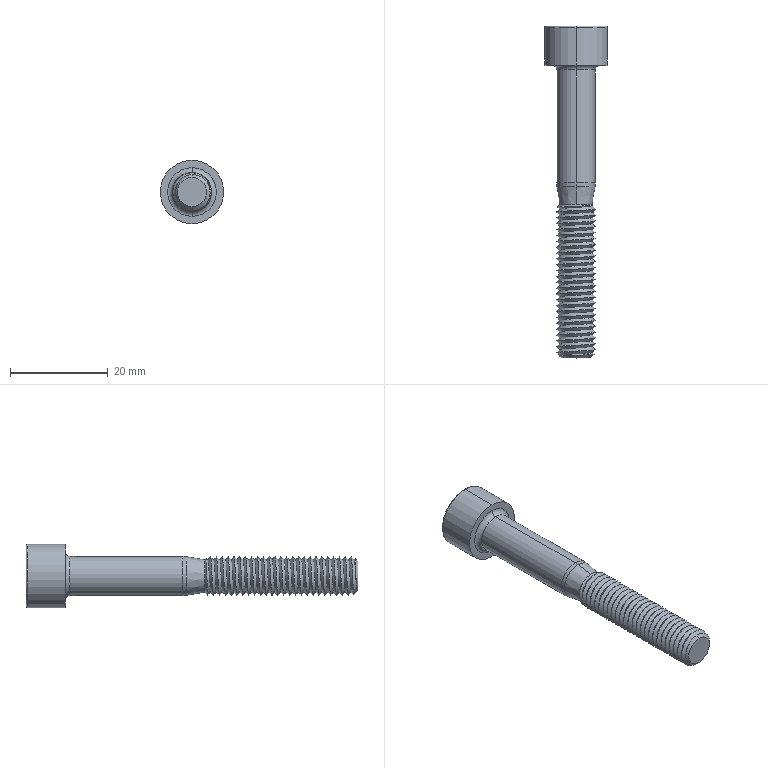Part | STEP file | Parafuso M8 - 60mm | 1 solid | 38 faces | box 13 x 68 x 13 mm | volume 3575 mm3 | plane 16 | cone 8 | torus 6 | cylinder 4 | other 2 | spline 2 | commonest cylinder face diameters 8 x2 13 x2